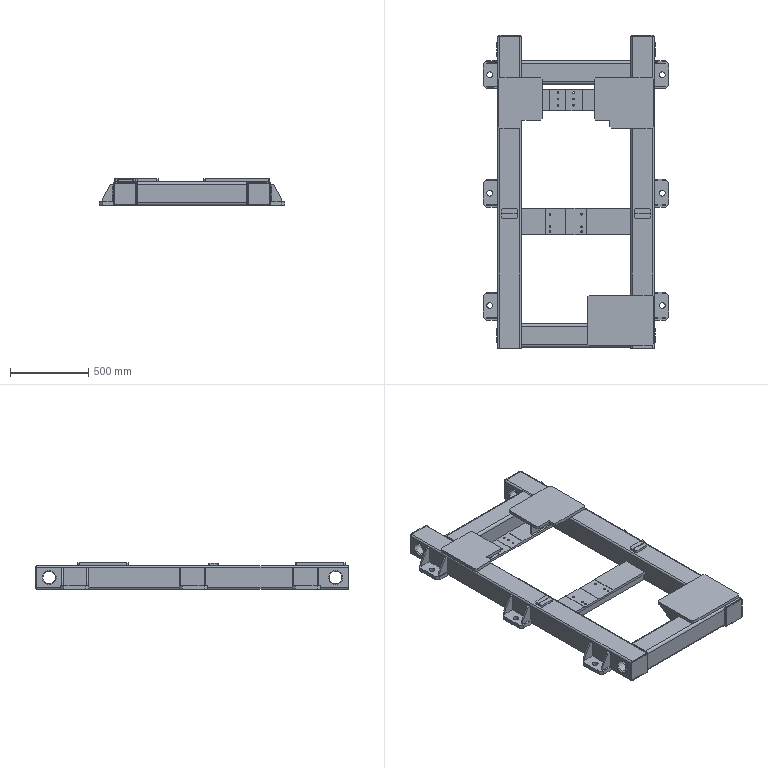Part | SolidWorks | features ICE 9, Boss 8, Chamfer 6, HoleWzd 5, LPattern 5, EndCap 4, Cut 2, MirrorSolid 1, WeldMemberFeat 1, WeldmentFeature 1 | 36 solids | 477 faces | box 1180 x 2000 x 170 mm | volume 41787721 mm3 | plane 375 | cylinder 102 | commonest cylinder face diameters 89 x24 12 x16 36 x12 4 x8 10.2 x8 16 x8